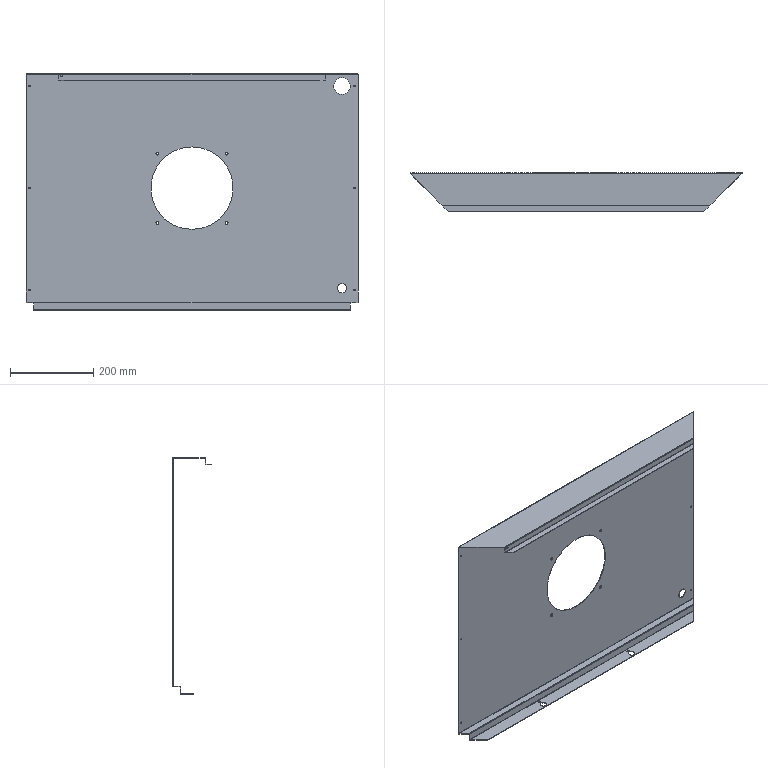Part | STEP file | HESS-408-70-15W-D-3-electrical box top plate | 1 solid | 96 faces | box 797 x 93.5 x 568.5 mm | volume 793198 mm3 | cylinder 50 | plane 34 | spline 12 | commonest cylinder face diameters 3.2 x18 7 x8 0.2 x6 4 x4 6 x4 5 x2